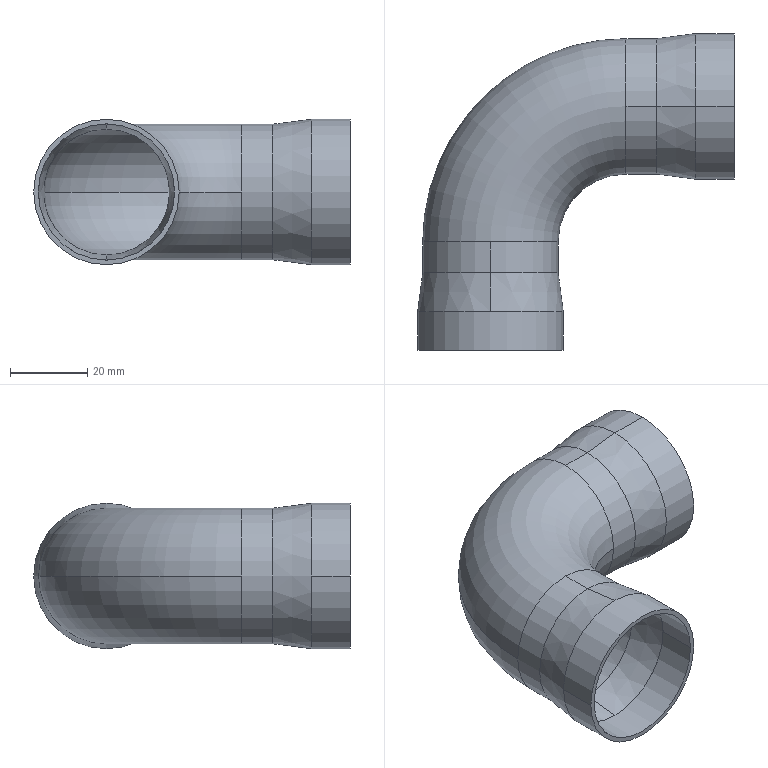Part | STEP file | right-angle cylinder elbow | 1 solid | 31 faces | box 81.8 x 81.8 x 37.6 mm | volume 14457 mm3 | cylinder 16 | cone 8 | torus 4 | plane 3 | commonest cylinder face diameters 32.6 x4 35 x4 35.2 x4 37.6 x4